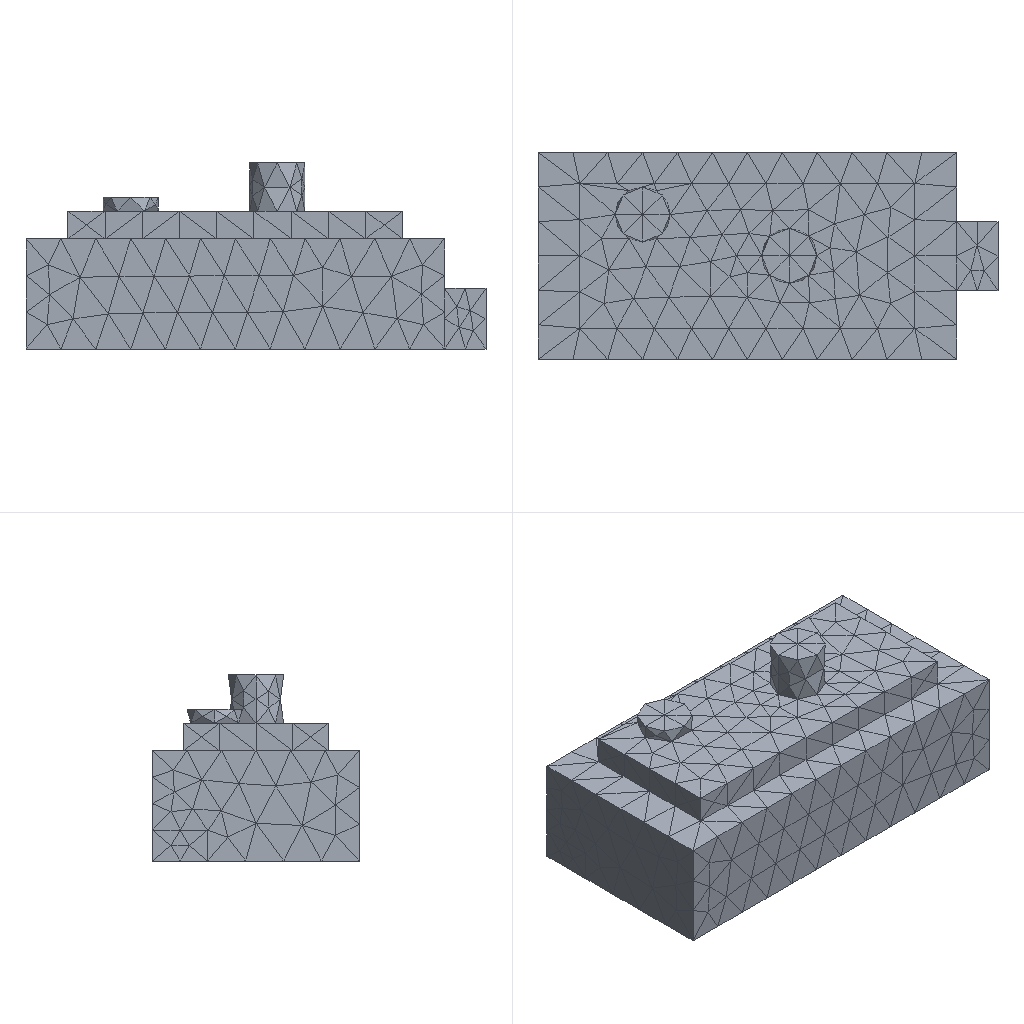Simulation study | ansys mapdl
Set-up summary:
category,name,step,type,value,unit,region
solver,ansys_mapdl
units,mm-N-s-tonne (MPa),,inferred,E=210000 density=
analysis,model,,static
mesh,nodes,,,4362
mesh,elements,,,2601
element_type,SOLID187,,,2601
material,mat 1,,E,210000
material,mat 1,,nu,0.3
load,,model,body load temp,,,all
load,,model,force,"1000 [dir=(0, 0, -1) n=123]",,node list
bc,,model,fixed,"[dofs=UX,UY,UZ n=4600]",,node list
Ansys APDL input file, long lists of numbers shortened:
/COM,ANSYS RELEASE 2026 R1           BUILD 26.1      UP20260202       09:09:40
/PREP7
/NOPR
/TITLE,2
ANTYPE, 0
*IF,_CDRDOFF,EQ,1,THEN     !if solid model was read in
_CDRDOFF=             !reset flag, numoffs already performed
*ELSE              !offset database for the following FE model
NUMOFF,NODE,     4362
NUMOFF,ELEM,     2601
NUMOFF,MAT ,        1
NUMOFF,TYPE,        1
*ENDIF
*SET,_RETURN ,  0.
*SET,_STATUS ,  0.
*SET,_UIQR   ,  123.
*SET,__FLOATPARAMETER__,  4362.
DOF,DELETE
ETBLOCK,        1,        1
(2i9,19a9)
        1      187        0        0        0        0        0        0        0        0        0        0        0        0        0        0        0        0        0        0        0
       -1
NBLOCK,6,SOLID,      4362,      4362
(3i9,6e21.13e3)
        1        0        0-4.4750000000000E+001 3.0000000000000E+001 9.0000000000000E+000
! (4361 more lines like these left out)
N,UNBL,LOC,       -1,
EBLOCK,19,SOLID,      2601,      2601
(19i10)
         1         1         1         1         0         0         0         0        10         0         1      1531       341      1683      1684      1932      1933      1934      1935
! (5201 more lines like these left out)
        -1
MPTEMP,UNBL, 1, 1,  0.    ,
MPDATA,UNBL, 1,EX  ,       1, 1,  210000.000    ,
MPTEMP,UNBL, 1, 1,  0.    ,
MPDATA,UNBL, 1,NUXY,       1, 1, 0.3    ,
MPTEMP,UNBL, 1, 1,  0.    ,
MPDATA,UNBL, 1,PRXY,       1, 1, 0.3    ,
EXTOPT,ATTR,      0,      0,      0
EXTOPT,ESIZE,  0,  0.
EXTOPT,ACLEAR,      0
TREF,  0.
IRLF,  0
BFUNIF,TEMP,_TINY
ACEL,  0.    ,  0.    ,  0.
OMEGA,  0.    ,  0.    ,  0.
DOMEGA,  0.    ,  0.    ,  0.
CGLOC,  0.    ,  0.    ,  0.
CGOMEGA,  0.    ,  0.    ,  0.
DCGOMG,  0.    ,  0.    ,  0.
KUSE,     0
TIME,  0.
ALPHAD,  0.
BETAD,  0.
DMPRAT,  0.
DMPSTR,  0.
CRPLIM, 0.1    ,   0
CRPLIM,  0.    ,   1
NCNV,     0, 1.000000000E+12,     0,  0.    ,  0.
NEQIT,     0
ERESX,DEFA
DBLOCK,      4600
(i9,a6,2(pg16.9))
        1  UX    0.00000000      0.00000000
! (4599 more lines like these left out)
       -1
FBLOCK,       123
(i9,a6,2(pg16.9))
      869  FZ   -8.13008130      0.00000000
! (122 more lines like these left out)
       -1
/GO
FINISH
Results summary:
result,analysis_type_db,,,static,unstated
result,n_sets,,,1,unstated
result,load_steps[0].set,load_step=1,,1,unstated
result,load_steps[0].substep,load_step=1,,1,unstated
result,load_steps[0].time,load_step=1,,1,unstated
result,load_steps[0].freq,load_step=1,,1,unstated
result,load_steps[0].max_usum,load_step=1,,0.0004906,unstated
result,load_steps[0].max_seqv,load_step=1,,5.924,unstated
result,load_steps[0].reaction_sum.FX,load_step=1,,1.10037e-11,unstated
result,load_steps[0].reaction_sum.FY,load_step=1,,-1.02408e-11,unstated
result,load_steps[0].reaction_sum.FZ,load_step=1,,1000,unstated
result,load_steps[0].reaction_sum.MX,load_step=1,,0,unstated
result,load_steps[0].reaction_sum.MY,load_step=1,,0,unstated
result,load_steps[0].reaction_sum.MZ,load_step=1,,0,unstated
result,convergence,,,results present for all listed sets,unstated